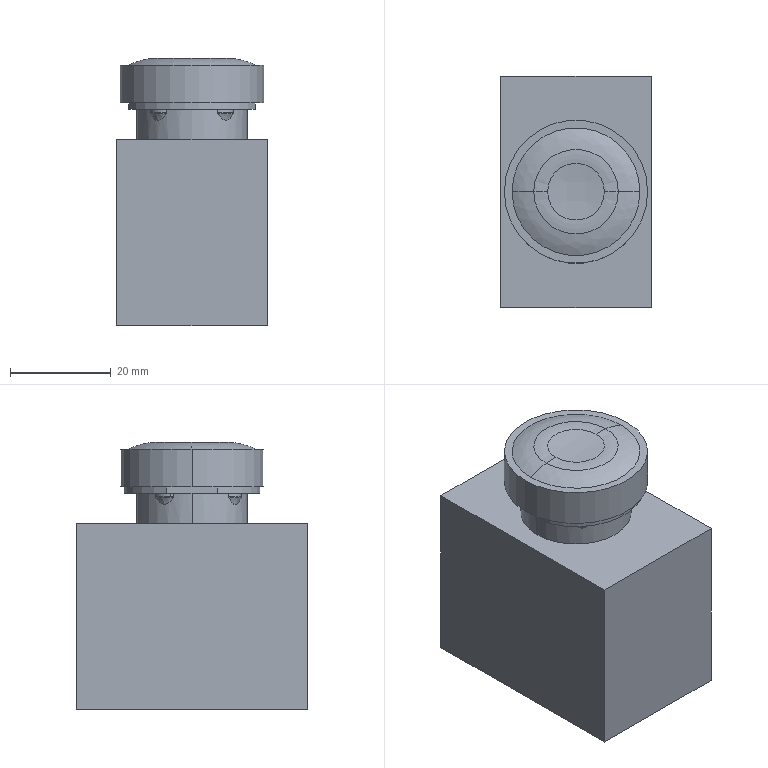Part | STEP file | ZBE-101-Y-1_1 | 1 solid | 69 faces | box 30 x 46 x 53.196 mm | volume 59289 mm3 | plane 28 | cylinder 22 | spline 13 | cone 6 | commonest cylinder face diameters 4.8 x4 6 x4 25.2 x4 0.7 x2 22 x2 27.15 x2